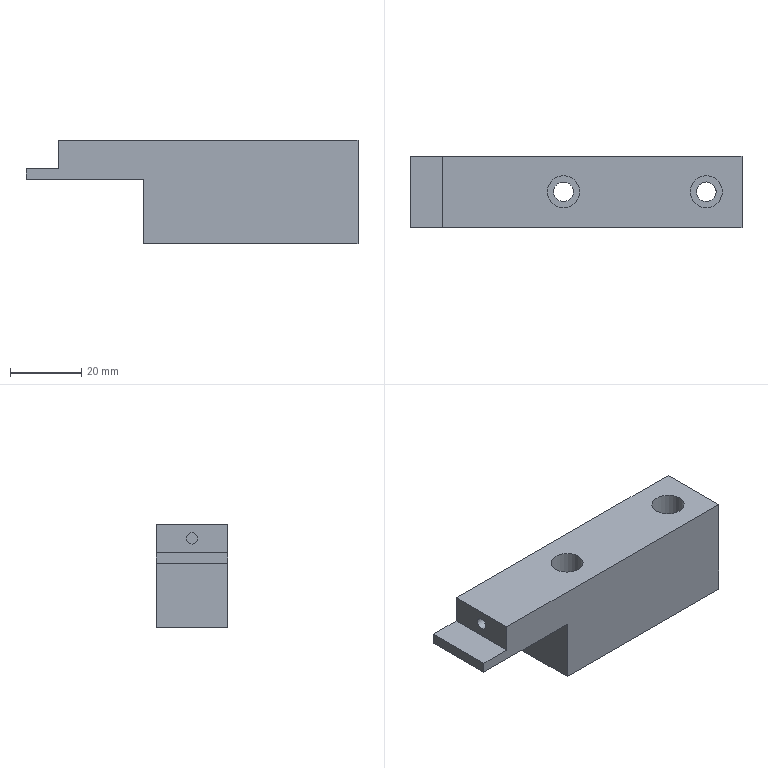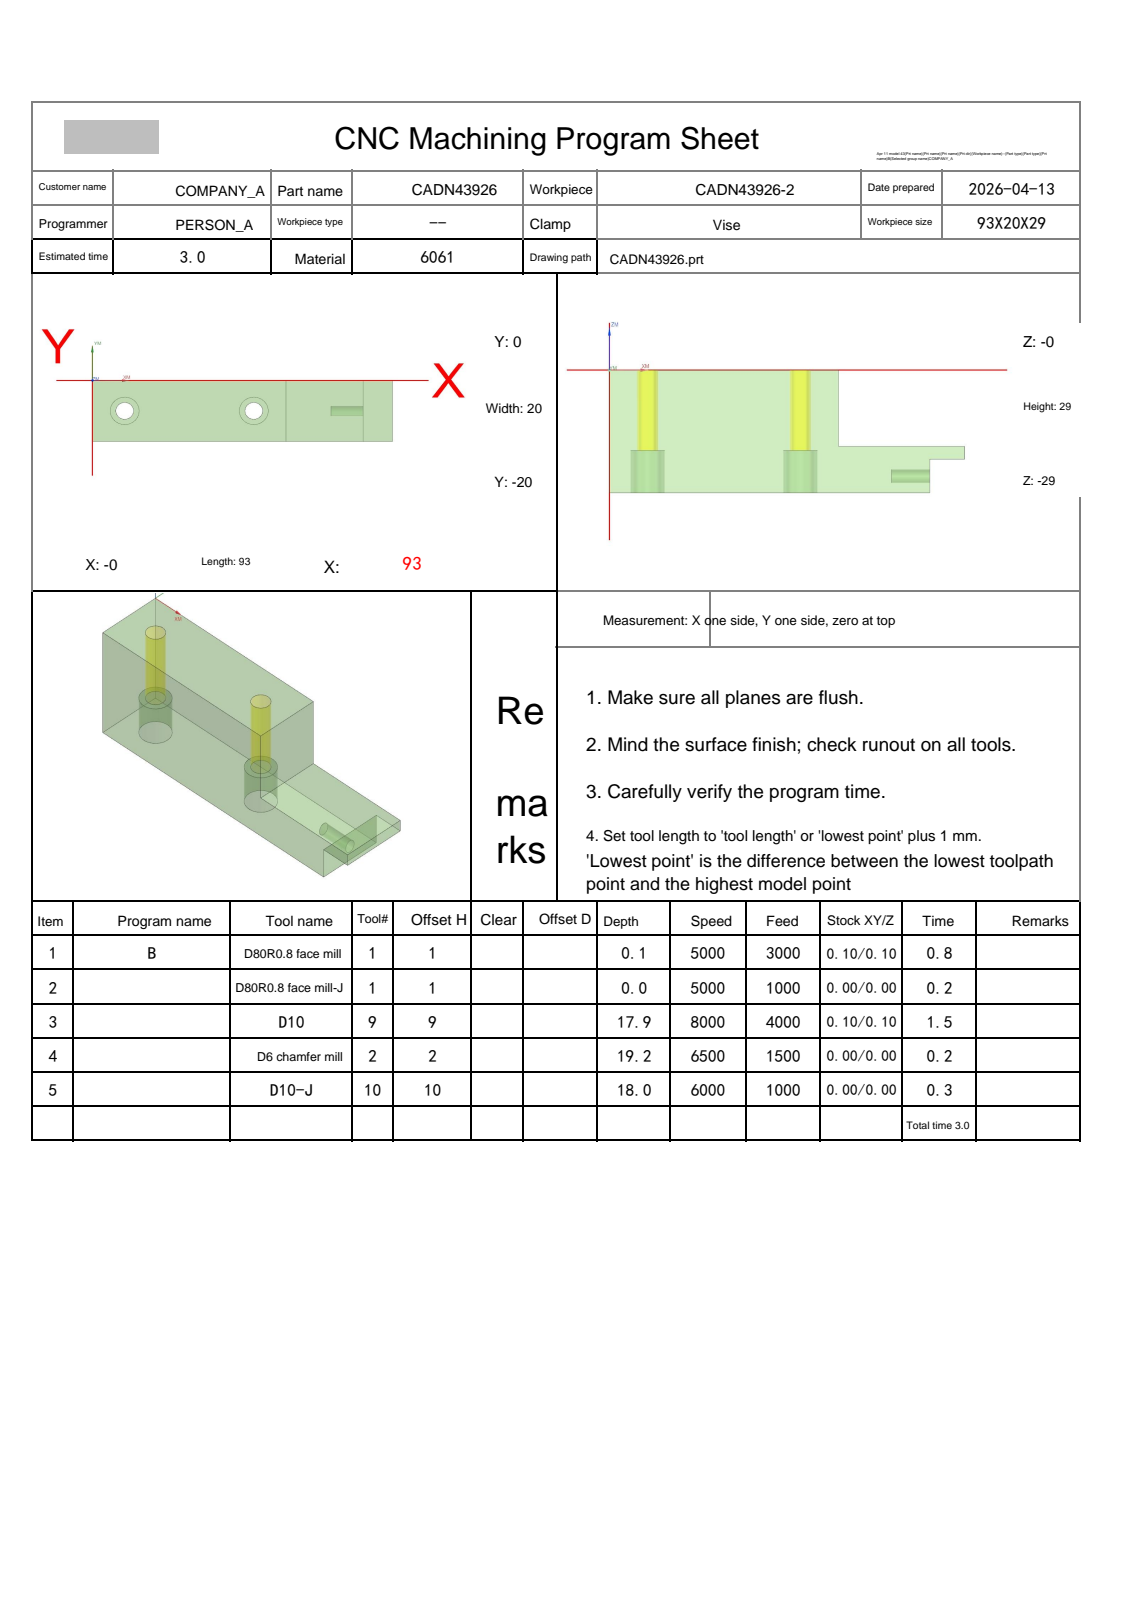NC program | NX | posted by the shop | part box 93 x 20 x 29 mm
Whole program:
%
O0001
(Machine time: 3.96 MIN)
(===Total Tool:4===)
(T1=D80R0.8 face mill D=80.  R=0.8  D-  H01 Z=0.    )
(T9=D10     D=10.  R=0.   D-  H09 Z=-17.9 )
(T2=D6 chamfer mill   D=6.   R=0.   D-  H02 Z=-19.2 )
(T10=D10-J  D=10.  R=0.   D10 H10 Z=-18.  )
G80 G90 G17 G49 G40
G91 G28 Z0
M01
N1 T01 M06
(D80R0.8 face mill  D=80. R=0.8 H=01 ce=0.10 di=0.10)
G00 G90 G54 X-52.097 Y-10. M03 S5000
G43 H01 Z20.
M08
Z6.011
G01 Z4.011 F3000.
X-40.097
X133.097
X145.097
Z6.011
G00 X-52.097
Z5.522
G01 Z3.522
X-40.097
X133.097
X145.097
Z5.522
G00 X-52.097
Z5.033
G01 Z3.033
X-40.097
X133.097
X145.097
Z5.033
G00 X-52.097
Z4.544
G01 Z2.544
X-40.097
X133.097
X145.097
Z4.544
G00 Z20.
X-52.097
Z4.056
G01 Z2.056
X-40.097
X133.097
X145.097
Z4.056
G00 Z20.
X-52.097
Z3.567
G01 Z1.567
X-40.097
X133.097
X145.097
Z3.567
G00 Z20.
X-52.097
Z3.078
G01 Z1.078
X-40.097
X133.097
X145.097
Z3.078
G00 Z20.
X-52.097
Z2.589
G01 Z.589
X-40.097
X133.097
X145.097
Z2.589
G00 Z20.
X-52.097
Z2.1
G01 Z.1
X-40.097
X133.097
X145.097
Z2.1
G00 Z20.
G91 G28 Z0.0
M05
M09
G91 G28 Z0.0
M01
N2 T01 M06
(D80R0.8 face mill-J  D=80. R=0.8 H=01 ce=0.00 di=0.00)
G00 G90 G54 X-51.999 Y-10. M03 S5000
G43 H01 Z20.
M08
Z2.
G01 Z0.0 F1000.
X-39.999
X132.999
X144.999
Z2.
G00 Z20.
G91 G28 Z0.0
M05
M09
G91 G28 Z0.0
M01
N3 T09 M06
(D10  D=10. R=0. H=09 ce=0.10 di=0.10)
G00 G90 G54 X95.1 Y8. M03 S8000
G43 H09 Z15.8
M08
Z.903
G01 Z-.597 F4000.
Y4.9
Y-23.9
G02 X94.1 Y-24.9 I-1. J0.0
G01 X93.
X88.6
G02 X87.6 Y-23.9 I0.0 J1.
G01 Y3.9
G03 X86.6 Y4.9 I-1. J0.0
G01 X81.1
G03 X80.1 Y3.9 I0.0 J-1.
G01 Y-23.9
G02 X79.1 Y-24.9 I-1. J0.0
G01 X73.6
G02 X72.6 Y-23.9 I0.0 J1.
G01 Y4.044
G03 X71.754 Y5.032 I-1. J0.0
G01 X66.254 Y5.888
X66.1 Y5.9
G03 X65.1 Y4.9 I0.0 J-1.
G01 Y-24.9
Y-28.1
Z.903
G00 X95.1 Y8.
Z.307
G01 Z-1.193
Y4.9
Y-23.9
G02 X94.1 Y-24.9 I-1. J0.0
G01 X93.
X88.6
G02 X87.6 Y-23.9 I0.0 J1.
G01 Y3.9
G03 X86.6 Y4.9 I-1. J0.0
G01 X81.1
G03 X80.1 Y3.9 I0.0 J-1.
G01 Y-23.9
G02 X79.1 Y-24.9 I-1. J0.0
G01 X73.6
G02 X72.6 Y-23.9 I0.0 J1.
G01 Y4.044
G03 X71.754 Y5.032 I-1. J0.0
G01 X66.254 Y5.888
X66.1 Y5.9
G03 X65.1 Y4.9 I0.0 J-1.
G01 Y-24.9
Y-28.1
Z.307
G00 X95.1 Y8.
Z-.29
G01 Z-1.79
Y4.9
Y-23.9
G02 X94.1 Y-24.9 I-1. J0.0
G01 X93.
X88.6
G02 X87.6 Y-23.9 I0.0 J1.
G01 Y3.9
G03 X86.6 Y4.9 I-1. J0.0
G01 X81.1
G03 X80.1 Y3.9 I0.0 J-1.
G01 Y-23.9
G02 X79.1 Y-24.9 I-1. J0.0
G01 X73.6
G02 X72.6 Y-23.9 I0.0 J1.
G01 Y4.044
G03 X71.754 Y5.032 I-1. J0.0
G01 X66.254 Y5.888
X66.1 Y5.9
G03 X65.1 Y4.9 I0.0 J-1.
G01 Y-24.9
Y-28.1
Z-.29
G00 X95.1 Y8.
Z-.887
G01 Z-2.387
Y4.9
Y-23.9
G02 X94.1 Y-24.9 I-1. J0.0
G01 X93.
X88.6
G02 X87.6 Y-23.9 I0.0 J1.
G01 Y3.9
G03 X86.6 Y4.9 I-1. J0.0
G01 X81.1
G03 X80.1 Y3.9 I0.0 J-1.
G01 Y-23.9
G02 X79.1 Y-24.9 I-1. J0.0
G01 X73.6
G02 X72.6 Y-23.9 I0.0 J1.
G01 Y4.044
G03 X71.754 Y5.032 I-1. J0.0
G01 X66.254 Y5.888
X66.1 Y5.9
G03 X65.1 Y4.9 I0.0 J-1.
G01 Y-24.9
Y-28.1
Z-.887
G00 X95.1 Y8.
Z-1.483
G01 Z-2.983
Y4.9
Y-23.9
G02 X94.1 Y-24.9 I-1. J0.0
G01 X93.
X88.6
G02 X87.6 Y-23.9 I0.0 J1.
G01 Y3.9
G03 X86.6 Y4.9 I-1. J0.0
G01 X81.1
G03 X80.1 Y3.9 I0.0 J-1.
G01 Y-23.9
G02 X79.1 Y-24.9 I-1. J0.0
G01 X73.6
G02 X72.6 Y-23.9 I0.0 J1.
G01 Y4.044
G03 X71.754 Y5.032 I-1. J0.0
G01 X66.254 Y5.888
X66.1 Y5.9
G03 X65.1 Y4.9 I0.0 J-1.
G01 Y-24.9
Y-28.1
Z-1.483
G00 X95.1 Y8.
Z-2.08
G01 Z-3.58
Y4.9
Y-23.9
G02 X94.1 Y-24.9 I-1. J0.0
G01 X93.
X88.6
G02 X87.6 Y-23.9 I0.0 J1.
G01 Y3.9
G03 X86.6 Y4.9 I-1. J0.0
G01 X81.1
G03 X80.1 Y3.9 I0.0 J-1.
G01 Y-23.9
G02 X79.1 Y-24.9 I-1. J0.0
G01 X73.6
G02 X72.6 Y-23.9 I0.0 J1.
G01 Y4.044
G03 X71.754 Y5.032 I-1. J0.0
G01 X66.254 Y5.888
X66.1 Y5.9
G03 X65.1 Y4.9 I0.0 J-1.
G01 Y-24.9
Y-28.1
Z-2.08
G00 X95.1 Y8.
Z-2.677
G01 Z-4.177
Y4.9
Y-23.9
G02 X94.1 Y-24.9 I-1. J0.0
G01 X93.
X88.6
G02 X87.6 Y-23.9 I0.0 J1.
G01 Y3.9
G03 X86.6 Y4.9 I-1. J0.0
G01 X81.1
G03 X80.1 Y3.9 I0.0 J-1.
G01 Y-23.9
G02 X79.1 Y-24.9 I-1. J0.0
G01 X73.6
G02 X72.6 Y-23.9 I0.0 J1.
G01 Y4.044
G03 X71.754 Y5.032 I-1. J0.0
G01 X66.254 Y5.888
X66.1 Y5.9
G03 X65.1 Y4.9 I0.0 J-1.
G01 Y-24.9
Y-28.1
Z-2.677
G00 X95.1 Y8.
Z-3.273
G01 Z-4.773
Y4.9
Y-23.9
G02 X94.1 Y-24.9 I-1. J0.0
G01 X93.
X88.6
G02 X87.6 Y-23.9 I0.0 J1.
G01 Y3.9
G03 X86.6 Y4.9 I-1. J0.0
G01 X81.1
G03 X80.1 Y3.9 I0.0 J-1.
G01 Y-23.9
G02 X79.1 Y-24.9 I-1. J0.0
G01 X73.6
G02 X72.6 Y-23.9 I0.0 J1.
G01 Y4.044
G03 X71.754 Y5.032 I-1. J0.0
G01 X66.254 Y5.888
X66.1 Y5.9
G03 X65.1 Y4.9 I0.0 J-1.
G01 Y-24.9
Y-28.1
Z-3.273
G00 X95.1 Y8.
Z-3.87
G01 Z-5.37
Y4.9
Y-23.9
G02 X94.1 Y-24.9 I-1. J0.0
G01 X93.
X88.6
G02 X87.6 Y-23.9 I0.0 J1.
G01 Y3.9
G03 X86.6 Y4.9 I-1. J0.0
G01 X81.1
G03 X80.1 Y3.9 I0.0 J-1.
G01 Y-23.9
G02 X79.1 Y-24.9 I-1. J0.0
G01 X73.6
G02 X72.6 Y-23.9 I0.0 J1.
G01 Y4.044
G03 X71.754 Y5.032 I-1. J0.0
G01 X66.254 Y5.888
X66.1 Y5.9
G03 X65.1 Y4.9 I0.0 J-1.
G01 Y-24.9
Y-28.1
Z-3.87
G00 X95.1 Y8.
Z-4.467
G01 Z-5.967
Y4.9
Y-23.9
G02 X94.1 Y-24.9 I-1. J0.0
G01 X93.
X88.6
G02 X87.6 Y-23.9 I0.0 J1.
G01 Y3.9
G03 X86.6 Y4.9 I-1. J0.0
G01 X81.1
G03 X80.1 Y3.9 I0.0 J-1.
G01 Y-23.9
G02 X79.1 Y-24.9 I-1. J0.0
G01 X73.6
G02 X72.6 Y-23.9 I0.0 J1.
G01 Y4.044
G03 X71.754 Y5.032 I-1. J0.0
G01 X66.254 Y5.888
X66.1 Y5.9
G03 X65.1 Y4.9 I0.0 J-1.
G01 Y-24.9
Y-28.1
Z-4.467
G00 X95.1 Y8.
Z-5.063
G01 Z-6.563
Y4.9
Y-23.9
G02 X94.1 Y-24.9 I-1. J0.0
G01 X93.
X88.6
G02 X87.6 Y-23.9 I0.0 J1.
G01 Y3.9
G03 X86.6 Y4.9 I-1. J0.0
G01 X81.1
G03 X80.1 Y3.9 I0.0 J-1.
G01 Y-23.9
G02 X79.1 Y-24.9 I-1. J0.0
G01 X73.6
G02 X72.6 Y-23.9 I0.0 J1.
G01 Y4.044
G03 X71.754 Y5.032 I-1. J0.0
G01 X66.254 Y5.888
X66.1 Y5.9
G03 X65.1 Y4.9 I0.0 J-1.
G01 Y-24.9
Y-28.1
Z-5.063
G00 X95.1 Y8.
Z-5.66
G01 Z-7.16
Y4.9
Y-23.9
G02 X94.1 Y-24.9 I-1. J0.0
G01 X93.
X88.6
G02 X87.6 Y-23.9 I0.0 J1.
G01 Y3.9
G03 X86.6 Y4.9 I-1. J0.0
G01 X81.1
G03 X80.1 Y3.9 I0.0 J-1.
G01 Y-23.9
G02 X79.1 Y-24.9 I-1. J0.0
G01 X73.6
G02 X72.6 Y-23.9 I0.0 J1.
G01 Y4.044
G03 X71.754 Y5.032 I-1. J0.0
G01 X66.254 Y5.888
X66.1 Y5.9
G03 X65.1 Y4.9 I0.0 J-1.
G01 Y-24.9
Y-28.1
Z-5.66
G00 X95.1 Y8.
Z-6.257
G01 Z-7.757
Y4.9
Y-23.9
G02 X94.1 Y-24.9 I-1. J0.0
G01 X93.
X88.6
G02 X87.6 Y-23.9 I0.0 J1.
G01 Y3.9
G03 X86.6 Y4.9 I-1. J0.0
G01 X81.1
G03 X80.1 Y3.9 I0.0 J-1.
G01 Y-23.9
G02 X79.1 Y-24.9 I-1. J0.0
G01 X73.6
G02 X72.6 Y-23.9 I0.0 J1.
G01 Y4.044
G03 X71.754 Y5.032 I-1. J0.0
G01 X66.254 Y5.888
X66.1 Y5.9
G03 X65.1 Y4.9 I0.0 J-1.
G01 Y-24.9
Y-28.1
Z-6.257
G00 X95.1 Y8.
Z-6.853
G01 Z-8.353
Y4.9
Y-23.9
G02 X94.1 Y-24.9 I-1. J0.0
G01 X93.
X88.6
G02 X87.6 Y-23.9 I0.0 J1.
G01 Y3.9
G03 X86.6 Y4.9 I-1. J0.0
G01 X81.1
G03 X80.1 Y3.9 I0.0 J-1.
G01 Y-23.9
G02 X79.1 Y-24.9 I-1. J0.0
G01 X73.6
G02 X72.6 Y-23.9 I0.0 J1.
G01 Y4.044
G03 X71.754 Y5.032 I-1. J0.0
G01 X66.254 Y5.888
X66.1 Y5.9
G03 X65.1 Y4.9 I0.0 J-1.
G01 Y-24.9
Y-28.1
Z-6.853
G00 X95.1 Y8.
Z-7.45
G01 Z-8.95
Y4.9
Y-23.9
G02 X94.1 Y-24.9 I-1. J0.0
G01 X93.
X88.6
G02 X87.6 Y-23.9 I0.0 J1.
G01 Y3.9
G03 X86.6 Y4.9 I-1. J0.0
G01 X81.1
G03 X80.1 Y3.9 I0.0 J-1.
G01 Y-23.9
G02 X79.1 Y-24.9 I-1. J0.0
G01 X73.6
G02 X72.6 Y-23.9 I0.0 J1.
G01 Y4.044
G03 X71.754 Y5.032 I-1. J0.0
G01 X66.254 Y5.888
X66.1 Y5.9
G03 X65.1 Y4.9 I0.0 J-1.
G01 Y-24.9
Y-28.1
Z-7.45
G00 X95.1 Y8.
Z-8.047
G01 Z-9.547
Y4.9
Y-23.9
G02 X94.1 Y-24.9 I-1. J0.0
G01 X93.
X88.6
G02 X87.6 Y-23.9 I0.0 J1.
G01 Y3.9
G03 X86.6 Y4.9 I-1. J0.0
G01 X81.1
G03 X80.1 Y3.9 I0.0 J-1.
G01 Y-23.9
G02 X79.1 Y-24.9 I-1. J0.0
G01 X73.6
G02 X72.6 Y-23.9 I0.0 J1.
G01 Y4.044
G03 X71.754 Y5.032 I-1. J0.0
G01 X66.254 Y5.888
X66.1 Y5.9
G03 X65.1 Y4.9 I0.0 J-1.
G01 Y-24.9
Y-28.1
Z-8.047
G00 X95.1 Y8.
Z-8.643
G01 Z-10.143
Y4.9
Y-23.9
G02 X94.1 Y-24.9 I-1. J0.0
G01 X93.
X88.6
G02 X87.6 Y-23.9 I0.0 J1.
G01 Y3.9
G03 X86.6 Y4.9 I-1. J0.0
G01 X81.1
G03 X80.1 Y3.9 I0.0 J-1.
G01 Y-23.9
G02 X79.1 Y-24.9 I-1. J0.0
G01 X73.6
G02 X72.6 Y-23.9 I0.0 J1.
G01 Y4.044
G03 X71.754 Y5.032 I-1. J0.0
G01 X66.254 Y5.888
X66.1 Y5.9
G03 X65.1 Y4.9 I0.0 J-1.
G01 Y-24.9
Y-28.1
Z-8.643
G00 X95.1 Y8.
Z-9.24
G01 Z-10.74
Y4.9
Y-23.9
G02 X94.1 Y-24.9 I-1. J0.0
G01 X93.
X88.6
G02 X87.6 Y-23.9 I0.0 J1.
G01 Y3.9
G03 X86.6 Y4.9 I-1. J0.0
G01 X81.1
G03 X80.1 Y3.9 I0.0 J-1.
G01 Y-23.9
G02 X79.1 Y-24.9 I-1. J0.0
G01 X73.6
G02 X72.6 Y-23.9 I0.0 J1.
G01 Y4.044
G03 X71.754 Y5.032 I-1. J0.0
G01 X66.254 Y5.888
X66.1 Y5.9
G03 X65.1 Y4.9 I0.0 J-1.
G01 Y-24.9
Y-28.1
Z-9.24
G00 X95.1 Y8.
Z-9.837
G01 Z-11.337
Y4.9
Y-23.9
G02 X94.1 Y-24.9 I-1. J0.0
G01 X93.
X88.6
G02 X87.6 Y-23.9 I0.0 J1.
G01 Y3.9
G03 X86.6 Y4.9 I-1. J0.0
G01 X81.1
G03 X80.1 Y3.9 I0.0 J-1.
G01 Y-23.9
G02 X79.1 Y-24.9 I-1. J0.0
G01 X73.6
G02 X72.6 Y-23.9 I0.0 J1.
G01 Y4.044
G03 X71.754 Y5.032 I-1. J0.0
G01 X66.254 Y5.888
X66.1 Y5.9
G03 X65.1 Y4.9 I0.0 J-1.
G01 Y-24.9
Y-28.1
Z-9.837
G00 X95.1 Y8.
Z-10.433
G01 Z-11.933
Y4.9
Y-23.9
G02 X94.1 Y-24.9 I-1. J0.0
G01 X93.
X88.6
G02 X87.6 Y-23.9 I0.0 J1.
G01 Y3.9
G03 X86.6 Y4.9 I-1. J0.0
G01 X81.1
G03 X80.1 Y3.9 I0.0 J-1.
G01 Y-23.9
G02 X79.1 Y-24.9 I-1. J0.0
G01 X73.6
G02 X72.6 Y-23.9 I0.0 J1.
G01 Y4.044
G03 X71.754 Y5.032 I-1. J0.0
G01 X66.254 Y5.888
X66.1 Y5.9
G03 X65.1 Y4.9 I0.0 J-1.
G01 Y-24.9
Y-28.1
Z-10.433
G00 X95.1 Y8.
Z-11.03
G01 Z-12.53
Y4.9
Y-23.9
G02 X94.1 Y-24.9 I-1. J0.0
G01 X93.
X88.6
G02 X87.6 Y-23.9 I0.0 J1.
G01 Y3.9
G03 X86.6 Y4.9 I-1. J0.0
G01 X81.1
G03 X80.1 Y3.9 I0.0 J-1.
G01 Y-23.9
G02 X79.1 Y-24.9 I-1. J0.0
G01 X73.6
G02 X72.6 Y-23.9 I0.0 J1.
G01 Y4.044
G03 X71.754 Y5.032 I-1. J0.0
G01 X66.254 Y5.888
X66.1 Y5.9
G03 X65.1 Y4.9 I0.0 J-1.
G01 Y-24.9
Y-28.1
Z-11.03
G00 X95.1 Y8.
Z-11.627
G01 Z-13.127
Y4.9
Y-23.9
G02 X94.1 Y-24.9 I-1. J0.0
G01 X93.
X88.6
G02 X87.6 Y-23.9 I0.0 J1.
G01 Y3.9
G03 X86.6 Y4.9 I-1. J0.0
G01 X81.1
G03 X80.1 Y3.9 I0.0 J-1.
G01 Y-23.9
G02 X79.1 Y-24.9 I-1. J0.0
G01 X73.6
G02 X72.6 Y-23.9 I0.0 J1.
G01 Y4.044
G03 X71.754 Y5.032 I-1. J0.0
G01 X66.254 Y5.888
X66.1 Y5.9
G03 X65.1 Y4.9 I0.0 J-1.
G01 Y-24.9
Y-28.1
Z-11.627
G00 X95.1 Y8.
Z-12.223
G01 Z-13.723
Y4.9
Y-23.9
G02 X94.1 Y-24.9 I-1. J0.0
G01 X93.
X88.6
G02 X87.6 Y-23.9 I0.0 J1.
G01 Y3.9
G03 X86.6 Y4.9 I-1. J0.0
G01 X81.1
G03 X80.1 Y3.9 I0.0 J-1.
G01 Y-23.9
G02 X79.1 Y-24.9 I-1. J0.0
G01 X73.6
G02 X72.6 Y-23.9 I0.0 J1.
G01 Y4.044
G03 X71.754 Y5.032 I-1. J0.0
G01 X66.254 Y5.888
X66.1 Y5.9
G03 X65.1 Y4.9 I0.0 J-1.
G01 Y-24.9
Y-28.1
Z-12.223
G00 X95.1 Y8.
Z-12.82
G01 Z-14.32
Y4.9
Y-23.9
G02 X94.1 Y-24.9 I-1. J0.0
G01 X93.
X88.6
G02 X87.6 Y-23.9 I0.0 J1.
G01 Y3.9
G03 X86.6 Y4.9 I-1. J0.0
G01 X81.1
G03 X80.1 Y3.9 I0.0 J-1.
G01 Y-23.9
G02 X79.1 Y-24.9 I-1. J0.0
G01 X73.6
G02 X72.6 Y-23.9 I0.0 J1.
G01 Y4.044
G03 X71.754 Y5.032 I-1. J0.0
G01 X66.254 Y5.888
X66.1 Y5.9
G03 X65.1 Y4.9 I0.0 J-1.
G01 Y-24.9
Y-28.1
Z-12.82
G00 X95.1 Y8.
Z-13.417
G01 Z-14.917
Y4.9
Y-23.9
G02 X94.1 Y-24.9 I-1. J0.0
G01 X93.
X88.6
G02 X87.6 Y-23.9 I0.0 J1.
G01 Y3.9
G03 X86.6 Y4.9 I-1. J0.0
G01 X81.1
G03 X80.1 Y3.9 I0.0 J-1.
G01 Y-23.9
G02 X79.1 Y-24.9 I-1. J0.0
G01 X73.6
G02 X72.6 Y-23.9 I0.0 J1.
G01 Y4.044
G03 X71.754 Y5.032 I-1. J0.0
G01 X66.254 Y5.888
X66.1 Y5.9
G03 X65.1 Y4.9 I0.0 J-1.
G01 Y-24.9
Y-28.1
Z-13.417
G00 X95.1 Y8.
Z-14.013
G01 Z-15.513
Y4.9
Y-23.9
G02 X94.1 Y-24.9 I-1. J0.0
G01 X93.
X88.6
G02 X87.6 Y-23.9 I0.0 J1.
G01 Y3.9
G03 X86.6 Y4.9 I-1. J0.0
G01 X81.1
G03 X80.1 Y3.9 I0.0 J-1.
G01 Y-23.9
G02 X79.1 Y-24.9 I-1. J0.0
G01 X73.6
G02 X72.6 Y-23.9 I0.0 J1.
G01 Y4.044
G03 X71.754 Y5.032 I-1. J0.0
G01 X66.254 Y5.888
X66.1 Y5.9
G03 X65.1 Y4.9 I0.0 J-1.
G01 Y-24.9
Y-28.1
Z-14.013
G00 X95.1 Y8.
Z-14.61
G01 Z-16.11
Y4.9
Y-23.9
G02 X94.1 Y-24.9 I-1. J0.0
G01 X93.
X88.6
G02 X87.6 Y-23.9 I0.0 J1.
G01 Y3.9
G03 X86.6 Y4.9 I-1. J0.0
G01 X81.1
G03 X80.1 Y3.9 I0.0 J-1.
G01 Y-23.9
G02 X79.1 Y-24.9 I-1. J0.0
G01 X73.6
G02 X72.6 Y-23.9 I0.0 J1.
G01 Y4.044
G03 X71.754 Y5.032 I-1. J0.0
G01 X66.254 Y5.888
X66.1 Y5.9
G03 X65.1 Y4.9 I0.0 J-1.
G01 Y-24.9
Y-28.1
Z-14.61
G00 X95.1 Y8.
Z-15.207
G01 Z-16.707
Y4.9
Y-23.9
G02 X94.1 Y-24.9 I-1. J0.0
G01 X93.
X88.6
G02 X87.6 Y-23.9 I0.0 J1.
G01 Y3.9
G03 X86.6 Y4.9 I-1. J0.0
G01 X81.1
G03 X80.1 Y3.9 I0.0 J-1.
G01 Y-23.9
G02 X79.1 Y-24.9 I-1. J0.0
G01 X73.6
G02 X72.6 Y-23.9 I0.0 J1.
G01 Y4.044
G03 X71.754 Y5.032 I-1. J0.0
G01 X66.254 Y5.888
X66.1 Y5.9
G03 X65.1 Y4.9 I0.0 J-1.
G01 Y-24.9
Y-28.1
Z-15.207
G00 X95.1 Y8.
Z-15.803
G01 Z-17.303
Y4.9
Y-23.9
G02 X94.1 Y-24.9 I-1. J0.0
G01 X93.
X88.6
G02 X87.6 Y-23.9 I0.0 J1.
G01 Y3.9
G03 X86.6 Y4.9 I-1. J0.0
G01 X81.1
G03 X80.1 Y3.9 I0.0 J-1.
G01 Y-23.9
G02 X79.1 Y-24.9 I-1. J0.0
G01 X73.6
G02 X72.6 Y-23.9 I0.0 J1.
G01 Y4.044
G03 X71.754 Y5.032 I-1. J0.0
G01 X66.254 Y5.888
X66.1 Y5.9
G03 X65.1 Y4.9 I0.0 J-1.
G01 Y-24.9
Y-28.1
Z-15.803
G00 X95.1 Y8.
Z-16.4
G01 Z-17.9
Y4.9
Y-23.9
G02 X94.1 Y-24.9 I-1. J0.0
G01 X93.
X88.6
G02 X87.6 Y-23.9 I0.0 J1.
G01 Y3.9
G03 X86.6 Y4.9 I-1. J0.0
G01 X81.1
G03 X80.1 Y3.9 I0.0 J-1.
G01 Y-23.9
G02 X79.1 Y-24.9 I-1. J0.0
G01 X73.6
G02 X72.6 Y-23.9 I0.0 J1.
G01 Y4.044
G03 X71.754 Y5.032 I-1. J0.0
G01 X66.254 Y5.888
X66.1 Y5.9
G03 X65.1 Y4.9 I0.0 J-1.
G01 Y-24.9
Y-28.1
Z-16.4
G00 Z15.8
G91 G28 Z0.0
M05
M09
G91 G28 Z0.0
M01
N4 T02 M06
(D6 chamfer mill  D=6. R=0. H=02 ce=0.00 di=0.00)
G00 G90 G54 X29.614 Y1.227 M03 S6500
G43 H02 Z20.
M08
Z.172
G01 Z-1.2 F1500.
G03 X29.9 Y1.027 I1.286 J1.532
G01 X29.946 Y.997
X30. Y1.
X60.
G02 X61. Y0.0 I0.0 J-1.
G01 Y-20.
G02 X60. Y-21. I-1. J0.0
G01 X0.0
G02 X-1. Y-20. I0.0 J1.
G01 Y0.0
G02 X0.0 Y1. I1. J0.0
G01 X30.
X30.054 Y.997
X30.1 Y1.027
G03 X30.386 Y1.227 I-1. J1.732
G01 Z.172
G00 Z10.
X48.435 Y-9.543
Z.275
G01 Z-1.2
G03 X48.266 Y-9.848 I1.658 J-1.118
G01 X48.241 Y-9.896
X48.25 Y-9.95
G03 X50. Y-11.7 I1.75 J0.0
X51.75 Y-9.95 I0.0 J1.75
X50. Y-8.2 I-1.75 J0.0
X48.25 Y-9.95 I0.0 J-1.75
G01 X48.241 Y-10.004
X48.266 Y-10.052
G03 X48.435 Y-10.357 I1.827 J.813
G01 Z.275
G00 Z10.
X11.565
Z.275
G01 Z-1.2
G03 X11.734 Y-10.052 I-1.658 J1.118
G01 X11.759 Y-10.004
X11.75 Y-9.95
G03 X10. Y-8.2 I-1.75 J0.0
X8.25 Y-9.95 I0.0 J-1.75
X10. Y-11.7 I1.75 J0.0
X11.75 Y-9.95 I0.0 J1.75
G01 X11.759 Y-9.896
X11.734 Y-9.848
G03 X11.565 Y-9.543 I-1.827 J-.813
G01 Z.275
G00 Z10.
X63.01 Y1.068
Z-1.795
G01 Z-19.2
X63.096 Y1.008
X63.126 Y1.
X93.
G02 X94. Y0.0 I0.0 J-1.
G01 Y-20.
G02 X93. Y-21. I-1. J0.0
G01 X63.126
X63.096 Y-21.008
X63.01 Y-21.068
Z-1.795
G00 Z20.
G91 G28 Z0.0
M05
M09
G91 G28 Z0.0
M01
N5 T10 M06
(D10-J  D=10. R=0. H=10 ce=0.40 di=0.00)
G00 G90 G54 X96. Y7. M03 S6000
G43 H10 Z15.8
M08
Z-16.5
G01 Z-18. F1000.
G03 X94. Y5. I0.0 J-2.
G01 Y-24.1
G02 X93.1 Y-25. I-.9 J0.0
G01 X90.233
G02 X89.233 Y-24. I0.0 J1.
G01 Y4.1
G03 X88.333 Y5. I-.9 J0.0
G01 X85.467
G03 X84.467 Y4. I0.0 J-1.
G01 Y-24.1
G02 X83.567 Y-25. I-.9 J0.0
G01 X80.7
G02 X79.7 Y-24. I0.0 J1.
G01 Y4.1
G03 X78.8 Y5. I-.9 J0.0
G01 X75.933
G03 X74.933 Y4. I0.0 J-1.
G01 Y-24.1
G02 X74.033 Y-25. I-.9 J0.0
G01 X71.167
G02 X70.167 Y-24. I0.0 J1.
G01 Y4.1
G03 X69.267 Y5. I-.9 J0.0
G01 X66.4
G03 X65.4 Y4. I0.0 J-1.
G01 Y-25.
G03 X67.4 Y-27. I2. J0.0
G01 Z-16.5
G00 Z15.8
G00 G90 X67.199 Y7. M03 S6000
Z15.8
Z-17.
G01 Z-18. F1000.
G41 D10
X66.999
G03 X65. Y5. I.001 J-2.
G01 Y-25.
G03 X67. Y-27. I2. J0.0
G01 G40 X67.2
Z-17.
G00 Z15.8
M05
M09
G91 G28 Z0.0
G91 G28 Y0.0
M30
%